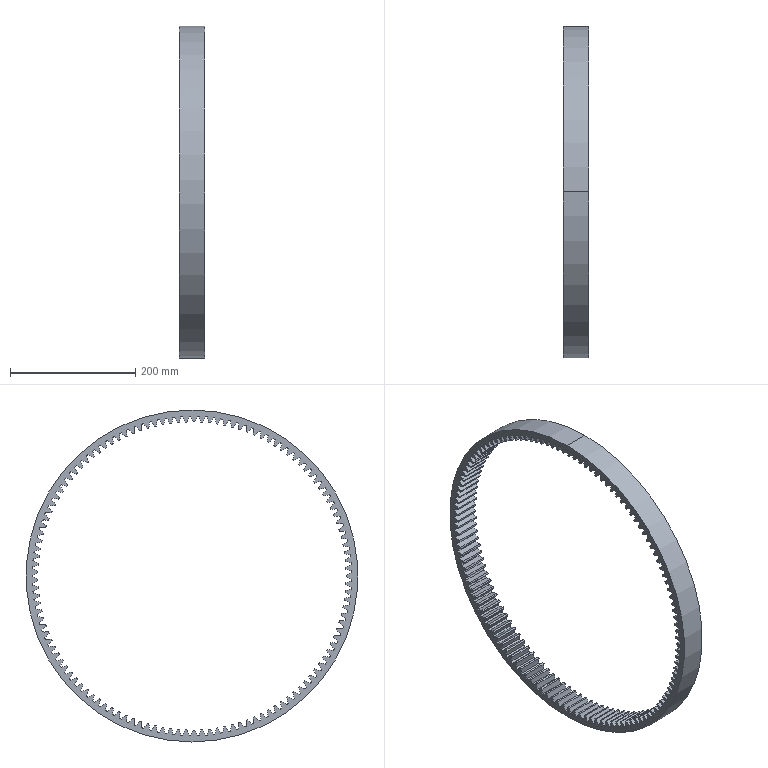Part | SolidWorks | features ICE 1, MBimport 1 | 1 solid | 507 faces | box 40 x 530 x 530 mm | volume 927581 mm3 | cylinder 505 | plane 2 | commonest cylinder face diameters 250 x253 492 x125 510.002 x125 530 x2